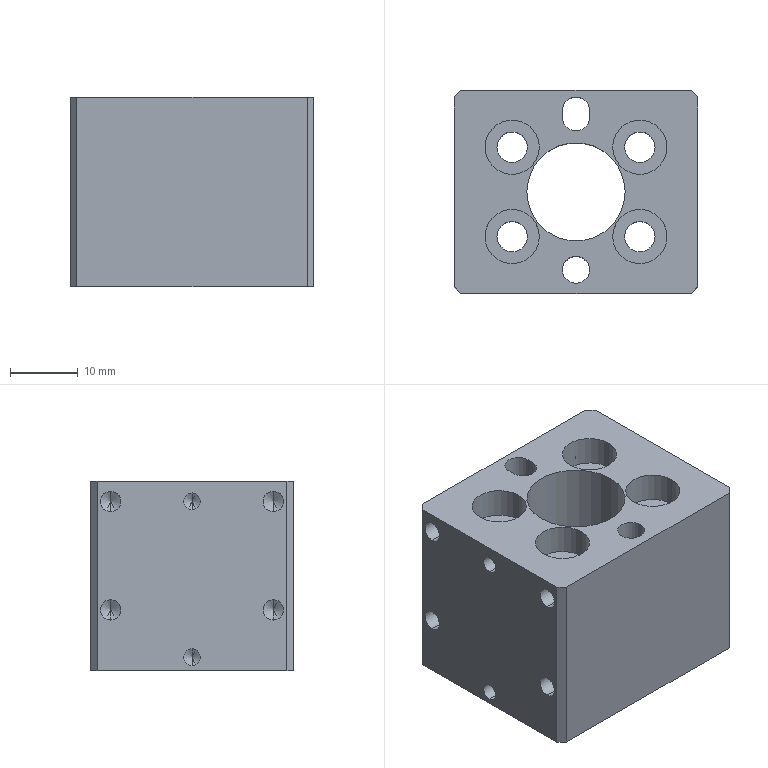Part | STEP file | 11-FG-SB00311 | 1 solid | 89 faces | box 36 x 30 x 28 mm | volume 21147 mm3 | cylinder 48 | cone 24 | plane 17 | commonest cylinder face diameters 3 x16 2.5 x8 4.5 x8 8 x8 4 x4 14.5 x2